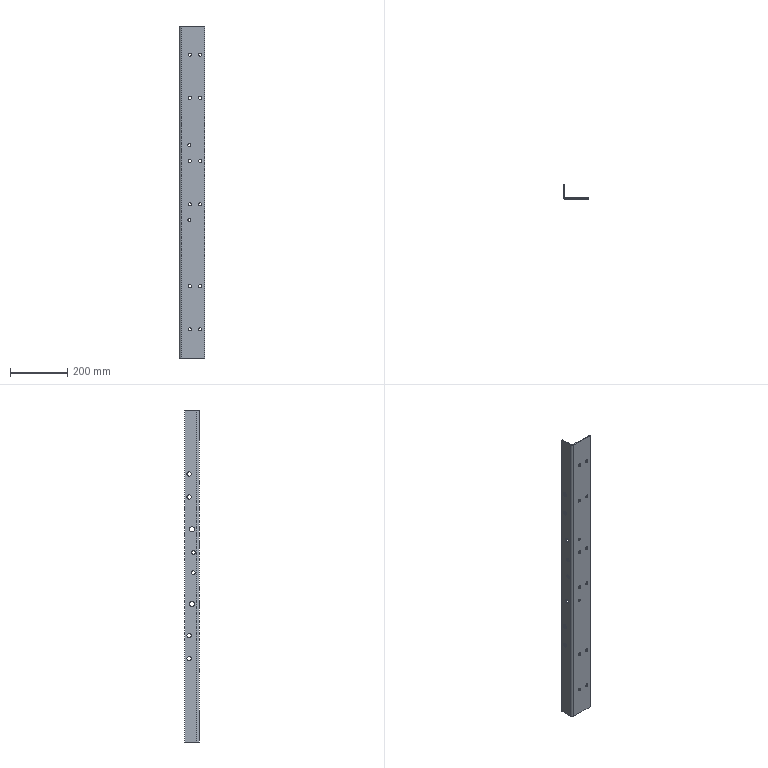Part | SolidWorks | features ICE 2, Chamfer 1, FlatPattern 1, MoveCopyBody 1, SMBaseFlange 1, SheetMetal 1 | 1 solid | 58 faces | box 88.5 x 50 x 1155 mm | volume 598465 mm3 | cylinder 46 | plane 12 | commonest cylinder face diameters 11 x28 15 x8 13 x4 17 x4 8 x1 16 x1